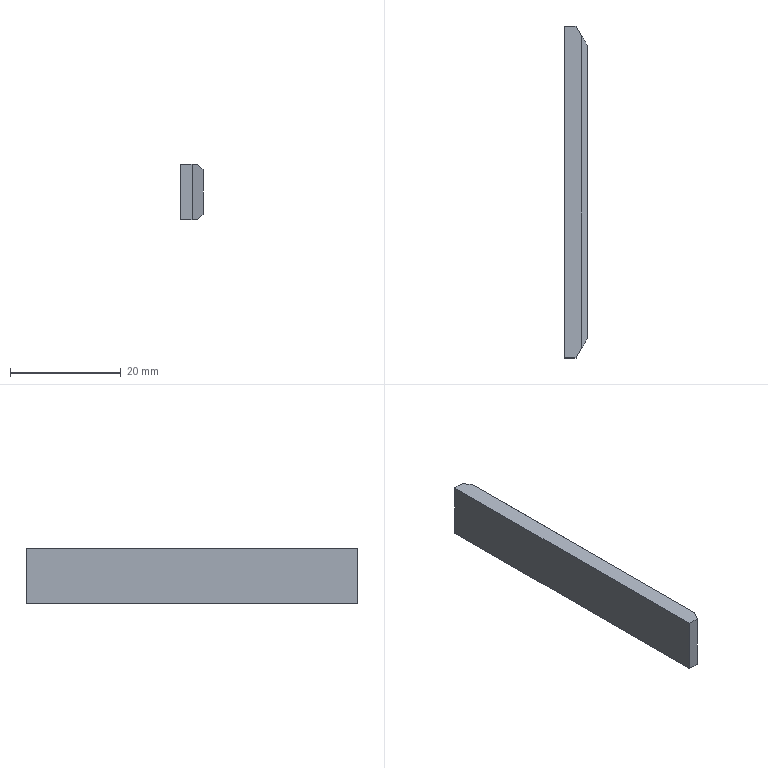Part | SolidWorks | features Chamfer 2, Extrusion 1 | 1 solid | 10 faces | box 4 x 60 x 10 mm | volume 2276 mm3 | plane 10
STEP:
#1=CARTESIAN_POINT('',(2.,-30.,5.));
#2=VERTEX_POINT('',#1);
#3=CARTESIAN_POINT('',(3.,-28.268,5.));
#4=VERTEX_POINT('',#3);
#5=CARTESIAN_POINT('',(4.,-26.536,5.));
#6=DIRECTION('',(0.5,0.866,0.));
#7=VECTOR('',#6,1000.);
#8=LINE('',#5,#7);
#9=EDGE_CURVE('',#2,#4,#8,.T.);
#10=ORIENTED_EDGE('',*,*,#9,.T.);
#11=CARTESIAN_POINT('',(3.,28.268,5.));
#12=VERTEX_POINT('',#11);
#13=CARTESIAN_POINT('',(3.,26.536,5.));
#14=DIRECTION('',(0.,1.,0.));
#15=VECTOR('',#14,1000.);
#16=LINE('',#13,#15);
#17=EDGE_CURVE('',#4,#12,#16,.T.);
#18=ORIENTED_EDGE('',*,*,#17,.T.);
#19=CARTESIAN_POINT('',(2.,30.,5.));
#20=VERTEX_POINT('',#19);
#21=CARTESIAN_POINT('',(4.,26.536,5.));
#22=DIRECTION('',(-0.5,0.866,0.));
#23=VECTOR('',#22,1000.);
#24=LINE('',#21,#23);
#25=EDGE_CURVE('',#12,#20,#24,.T.);
#26=ORIENTED_EDGE('',*,*,#25,.T.);
#27=CARTESIAN_POINT('',(0.,30.,5.));
#28=VERTEX_POINT('',#27);
#29=CARTESIAN_POINT('',(4.,30.,5.));
#30=DIRECTION('',(-1.,0.,0.));
#31=VECTOR('',#30,1000.);
#32=LINE('',#29,#31);
#33=EDGE_CURVE('',#20,#28,#32,.T.);
#34=ORIENTED_EDGE('',*,*,#33,.T.);
#35=CARTESIAN_POINT('',(0.,-30.,5.));
#36=VERTEX_POINT('',#35);
#37=CARTESIAN_POINT('',(0.,-30.,5.));
#38=DIRECTION('',(0.,-1.,0.));
#39=VECTOR('',#38,1000.);
#40=LINE('',#37,#39);
#41=EDGE_CURVE('',#28,#36,#40,.T.);
#42=ORIENTED_EDGE('',*,*,#41,.T.);
#43=CARTESIAN_POINT('',(4.,-30.,5.));
#44=DIRECTION('',(-1.,0.,0.));
#45=VECTOR('',#44,1000.);
#46=LINE('',#43,#45);
#47=EDGE_CURVE('',#2,#36,#46,.T.);
#48=ORIENTED_EDGE('',*,*,#47,.F.);
#49=EDGE_LOOP('',(#10,#18,#26,#34,#42,#48));
#50=FACE_OUTER_BOUND('',#49,.T.);
#51=CARTESIAN_POINT('',(4.,-30.,5.));
#52=DIRECTION('',(0.,0.,-1.));
#53=DIRECTION('',(-1.,0.,0.));
#54=AXIS2_PLACEMENT_3D('',#51,#52,#53);
#55=PLANE('',#54);
#56=ADVANCED_FACE('',(#50),#55,.F.);
#57=CARTESIAN_POINT('',(2.,-30.,-5.));
#58=VERTEX_POINT('',#57);
#59=CARTESIAN_POINT('',(0.,-30.,-5.));
#60=VERTEX_POINT('',#59);
#61=CARTESIAN_POINT('',(4.,-30.,-5.));
#62=DIRECTION('',(-1.,0.,0.));
#63=VECTOR('',#62,1000.);
#64=LINE('',#61,#63);
#65=EDGE_CURVE('',#58,#60,#64,.T.);
#66=ORIENTED_EDGE('',*,*,#65,.F.);
#67=CARTESIAN_POINT('',(2.,-30.,5.));
#68=DIRECTION('',(0.,0.,1.));
#69=VECTOR('',#68,1000.);
#70=LINE('',#67,#69);
#71=EDGE_CURVE('',#58,#2,#70,.T.);
#72=ORIENTED_EDGE('',*,*,#71,.T.);
#73=ORIENTED_EDGE('',*,*,#47,.T.);
#74=CARTESIAN_POINT('',(0.,-30.,-5.));
#75=DIRECTION('',(0.,0.,-1.));
#76=VECTOR('',#75,1000.);
#77=LINE('',#74,#76);
#78=EDGE_CURVE('',#36,#60,#77,.T.);
#79=ORIENTED_EDGE('',*,*,#78,.T.);
#80=EDGE_LOOP('',(#66,#72,#73,#79));
#81=FACE_OUTER_BOUND('',#80,.T.);
#82=CARTESIAN_POINT('',(4.,-30.,-5.));
#83=DIRECTION('',(0.,1.,0.));
#84=DIRECTION('',(0.,0.,1.));
#85=AXIS2_PLACEMENT_3D('',#82,#83,#84);
#86=PLANE('',#85);
#87=ADVANCED_FACE('',(#81),#86,.F.);
#88=CARTESIAN_POINT('',(2.,30.,-5.));
#89=VERTEX_POINT('',#88);
#90=CARTESIAN_POINT('',(3.,28.268,-5.));
#91=VERTEX_POINT('',#90);
#92=CARTESIAN_POINT('',(4.,26.536,-5.));
#93=DIRECTION('',(0.5,-0.866,0.));
#94=VECTOR('',#93,1000.);
#95=LINE('',#92,#94);
#96=EDGE_CURVE('',#89,#91,#95,.T.);
#97=ORIENTED_EDGE('',*,*,#96,.T.);
#98=CARTESIAN_POINT('',(3.,-28.268,-5.));
#99=VERTEX_POINT('',#98);
#100=CARTESIAN_POINT('',(3.,-26.536,-5.));
#101=DIRECTION('',(0.,-1.,0.));
#102=VECTOR('',#101,1000.);
#103=LINE('',#100,#102);
#104=EDGE_CURVE('',#91,#99,#103,.T.);
#105=ORIENTED_EDGE('',*,*,#104,.T.);
#106=CARTESIAN_POINT('',(4.,-26.536,-5.));
#107=DIRECTION('',(-0.5,-0.866,0.));
#108=VECTOR('',#107,1000.);
#109=LINE('',#106,#108);
#110=EDGE_CURVE('',#99,#58,#109,.T.);
#111=ORIENTED_EDGE('',*,*,#110,.T.);
#112=ORIENTED_EDGE('',*,*,#65,.T.);
#113=CARTESIAN_POINT('',(0.,30.,-5.));
#114=VERTEX_POINT('',#113);
#115=CARTESIAN_POINT('',(0.,-30.,-5.));
#116=DIRECTION('',(0.,1.,0.));
#117=VECTOR('',#116,1000.);
#118=LINE('',#115,#117);
#119=EDGE_CURVE('',#60,#114,#118,.T.);
#120=ORIENTED_EDGE('',*,*,#119,.T.);
#121=CARTESIAN_POINT('',(4.,30.,-5.));
#122=DIRECTION('',(-1.,0.,0.));
#123=VECTOR('',#122,1000.);
#124=LINE('',#121,#123);
#125=EDGE_CURVE('',#89,#114,#124,.T.);
#126=ORIENTED_EDGE('',*,*,#125,.F.);
#127=EDGE_LOOP('',(#97,#105,#111,#112,#120,#126));
#128=FACE_OUTER_BOUND('',#127,.T.);
#129=CARTESIAN_POINT('',(4.,-30.,-5.));
#130=DIRECTION('',(0.,0.,1.));
#131=DIRECTION('',(1.,0.,0.));
#132=AXIS2_PLACEMENT_3D('',#129,#130,#131);
#133=PLANE('',#132);
#134=ADVANCED_FACE('',(#128),#133,.F.);
#135=ORIENTED_EDGE('',*,*,#33,.F.);
#136=CARTESIAN_POINT('',(2.,30.,-5.));
#137=DIRECTION('',(0.,0.,-1.));
#138=VECTOR('',#137,1000.);
#139=LINE('',#136,#138);
#140=EDGE_CURVE('',#20,#89,#139,.T.);
#141=ORIENTED_EDGE('',*,*,#140,.T.);
#142=ORIENTED_EDGE('',*,*,#125,.T.);
#143=CARTESIAN_POINT('',(0.,30.,-5.));
#144=DIRECTION('',(0.,0.,1.));
#145=VECTOR('',#144,1000.);
#146=LINE('',#143,#145);
#147=EDGE_CURVE('',#114,#28,#146,.T.);
#148=ORIENTED_EDGE('',*,*,#147,.T.);
#149=EDGE_LOOP('',(#135,#141,#142,#148));
#150=FACE_OUTER_BOUND('',#149,.T.);
#151=CARTESIAN_POINT('',(4.,30.,-5.));
#152=DIRECTION('',(0.,-1.,0.));
#153=DIRECTION('',(0.,0.,-1.));
#154=AXIS2_PLACEMENT_3D('',#151,#152,#153);
#155=PLANE('',#154);
#156=ADVANCED_FACE('',(#150),#155,.F.);
#157=CARTESIAN_POINT('',(4.,-26.536,4.));
#158=VERTEX_POINT('',#157);
#159=CARTESIAN_POINT('',(4.,-26.536,-4.));
#160=VERTEX_POINT('',#159);
#161=CARTESIAN_POINT('',(4.,-26.536,-5.));
#162=DIRECTION('',(0.,0.,-1.));
#163=VECTOR('',#162,1000.);
#164=LINE('',#161,#163);
#165=EDGE_CURVE('',#158,#160,#164,.T.);
#166=ORIENTED_EDGE('',*,*,#165,.T.);
#167=CARTESIAN_POINT('',(4.,26.536,-4.));
#168=VERTEX_POINT('',#167);
#169=CARTESIAN_POINT('',(4.,26.536,-4.));
#170=DIRECTION('',(0.,1.,0.));
#171=VECTOR('',#170,1000.);
#172=LINE('',#169,#171);
#173=EDGE_CURVE('',#160,#168,#172,.T.);
#174=ORIENTED_EDGE('',*,*,#173,.T.);
#175=CARTESIAN_POINT('',(4.,26.536,4.));
#176=VERTEX_POINT('',#175);
#177=CARTESIAN_POINT('',(4.,26.536,5.));
#178=DIRECTION('',(0.,0.,1.));
#179=VECTOR('',#178,1000.);
#180=LINE('',#177,#179);
#181=EDGE_CURVE('',#168,#176,#180,.T.);
#182=ORIENTED_EDGE('',*,*,#181,.T.);
#183=CARTESIAN_POINT('',(4.,-26.536,4.));
#184=DIRECTION('',(0.,-1.,0.));
#185=VECTOR('',#184,1000.);
#186=LINE('',#183,#185);
#187=EDGE_CURVE('',#176,#158,#186,.T.);
#188=ORIENTED_EDGE('',*,*,#187,.T.);
#189=EDGE_LOOP('',(#166,#174,#182,#188));
#190=FACE_OUTER_BOUND('',#189,.T.);
#191=CARTESIAN_POINT('',(4.,0.,0.));
#192=DIRECTION('',(1.,0.,0.));
#193=DIRECTION('',(0.,0.,-1.));
#194=AXIS2_PLACEMENT_3D('',#191,#192,#193);
#195=PLANE('',#194);
#196=ADVANCED_FACE('',(#190),#195,.T.);
#197=ORIENTED_EDGE('',*,*,#41,.F.);
#198=ORIENTED_EDGE('',*,*,#147,.F.);
#199=ORIENTED_EDGE('',*,*,#119,.F.);
#200=ORIENTED_EDGE('',*,*,#78,.F.);
#201=EDGE_LOOP('',(#197,#198,#199,#200));
#202=FACE_OUTER_BOUND('',#201,.T.);
#203=CARTESIAN_POINT('',(0.,0.,0.));
#204=DIRECTION('',(1.,0.,0.));
#205=DIRECTION('',(0.,0.,-1.));
#206=AXIS2_PLACEMENT_3D('',#203,#204,#205);
#207=PLANE('',#206);
#208=ADVANCED_FACE('',(#202),#207,.F.);
#209=ORIENTED_EDGE('',*,*,#110,.F.);
#210=CARTESIAN_POINT('',(4.8,-25.15,-3.2));
#211=DIRECTION('',(0.4472,0.7746,0.4472));
#212=VECTOR('',#211,1000.);
#213=LINE('',#210,#212);
#214=EDGE_CURVE('',#99,#160,#213,.T.);
#215=ORIENTED_EDGE('',*,*,#214,.T.);
#216=ORIENTED_EDGE('',*,*,#165,.F.);
#217=CARTESIAN_POINT('',(4.8,-25.15,3.2));
#218=DIRECTION('',(-0.4472,-0.7746,0.4472));
#219=VECTOR('',#218,1000.);
#220=LINE('',#217,#219);
#221=EDGE_CURVE('',#158,#4,#220,.T.);
#222=ORIENTED_EDGE('',*,*,#221,.T.);
#223=ORIENTED_EDGE('',*,*,#9,.F.);
#224=ORIENTED_EDGE('',*,*,#71,.F.);
#225=EDGE_LOOP('',(#209,#215,#216,#222,#223,#224));
#226=FACE_OUTER_BOUND('',#225,.T.);
#227=CARTESIAN_POINT('',(4.,-26.536,0.));
#228=DIRECTION('',(0.866,-0.5,0.));
#229=DIRECTION('',(0.,0.,1.));
#230=AXIS2_PLACEMENT_3D('',#227,#228,#229);
#231=PLANE('',#230);
#232=ADVANCED_FACE('',(#226),#231,.T.);
#233=ORIENTED_EDGE('',*,*,#181,.F.);
#234=CARTESIAN_POINT('',(4.8,25.15,-3.2));
#235=DIRECTION('',(-0.4472,0.7746,-0.4472));
#236=VECTOR('',#235,1000.);
#237=LINE('',#234,#236);
#238=EDGE_CURVE('',#168,#91,#237,.T.);
#239=ORIENTED_EDGE('',*,*,#238,.T.);
#240=ORIENTED_EDGE('',*,*,#96,.F.);
#241=ORIENTED_EDGE('',*,*,#140,.F.);
#242=ORIENTED_EDGE('',*,*,#25,.F.);
#243=CARTESIAN_POINT('',(4.8,25.15,3.2));
#244=DIRECTION('',(0.4472,-0.7746,-0.4472));
#245=VECTOR('',#244,1000.);
#246=LINE('',#243,#245);
#247=EDGE_CURVE('',#12,#176,#246,.T.);
#248=ORIENTED_EDGE('',*,*,#247,.T.);
#249=EDGE_LOOP('',(#233,#239,#240,#241,#242,#248));
#250=FACE_OUTER_BOUND('',#249,.T.);
#251=CARTESIAN_POINT('',(4.,26.536,0.));
#252=DIRECTION('',(0.866,0.5,0.));
#253=DIRECTION('',(0.,0.,-1.));
#254=AXIS2_PLACEMENT_3D('',#251,#252,#253);
#255=PLANE('',#254);
#256=ADVANCED_FACE('',(#250),#255,.T.);
#257=ORIENTED_EDGE('',*,*,#214,.F.);
#258=ORIENTED_EDGE('',*,*,#104,.F.);
#259=ORIENTED_EDGE('',*,*,#238,.F.);
#260=ORIENTED_EDGE('',*,*,#173,.F.);
#261=EDGE_LOOP('',(#257,#258,#259,#260));
#262=FACE_OUTER_BOUND('',#261,.T.);
#263=CARTESIAN_POINT('',(4.,0.,-4.));
#264=DIRECTION('',(0.7071,0.,-0.7071));
#265=DIRECTION('',(0.,-1.,0.));
#266=AXIS2_PLACEMENT_3D('',#263,#264,#265);
#267=PLANE('',#266);
#268=ADVANCED_FACE('',(#262),#267,.T.);
#269=ORIENTED_EDGE('',*,*,#247,.F.);
#270=ORIENTED_EDGE('',*,*,#17,.F.);
#271=ORIENTED_EDGE('',*,*,#221,.F.);
#272=ORIENTED_EDGE('',*,*,#187,.F.);
#273=EDGE_LOOP('',(#269,#270,#271,#272));
#274=FACE_OUTER_BOUND('',#273,.T.);
#275=CARTESIAN_POINT('',(4.,0.,4.));
#276=DIRECTION('',(0.7071,0.,0.7071));
#277=DIRECTION('',(0.,1.,0.));
#278=AXIS2_PLACEMENT_3D('',#275,#276,#277);
#279=PLANE('',#278);
#280=ADVANCED_FACE('',(#274),#279,.T.);
#281=CLOSED_SHELL('',(#56,#87,#134,#156,#196,#208,#232,#256,#268,#280));
#282=MANIFOLD_SOLID_BREP('',#281);
#283=CARTESIAN_POINT('',(0.,0.,0.));
#284=DIRECTION('',(0.,0.,1.));
#285=DIRECTION('',(1.,0.,0.));
#286=AXIS2_PLACEMENT_3D('',#283,#284,#285);
#287=(LENGTH_UNIT()NAMED_UNIT(*)SI_UNIT(.MILLI.,.METRE.));
#288=UNCERTAINTY_MEASURE_WITH_UNIT(LENGTH_MEASURE(0.00001),#287,'','');
#289=(NAMED_UNIT(*)PLANE_ANGLE_UNIT()SI_UNIT($,.RADIAN.));
#290=(NAMED_UNIT(*)SI_UNIT($,.STERADIAN.)SOLID_ANGLE_UNIT());
#291=(GEOMETRIC_REPRESENTATION_CONTEXT(3)GLOBAL_UNCERTAINTY_ASSIGNED_CONTEXT((#288))GLOBAL_UNIT_ASSIGNED_CONTEXT((#287,#289,#290))REPRESENTATION_CONTEXT('',''));
#292=ADVANCED_BREP_SHAPE_REPRESENTATION('',(#282,#286),#291);